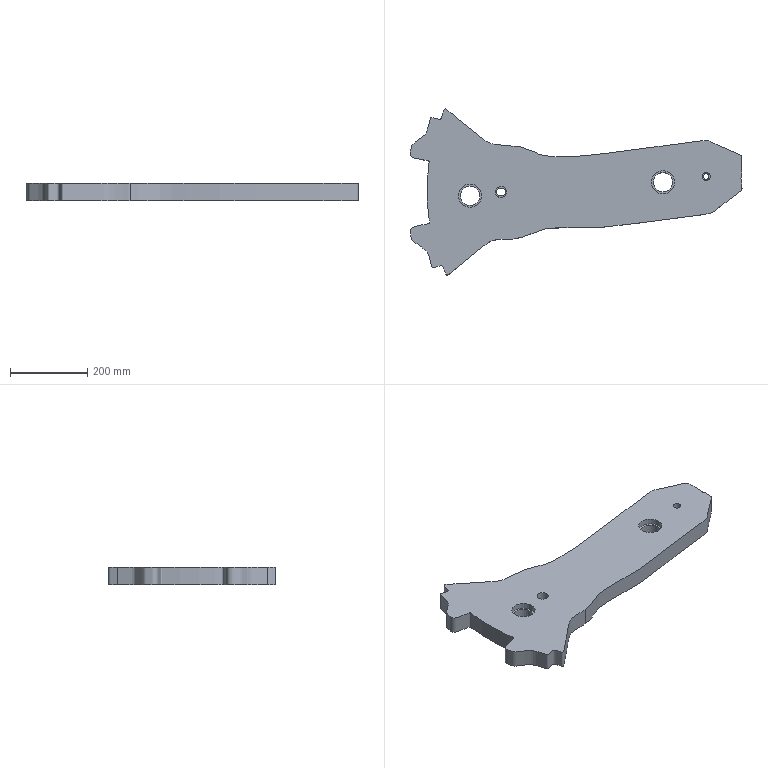Part | NX | features solid 2 | 1 solid | 29 faces | box 860.43 x 430.677 x 45 mm | volume 8766839 mm3 | cylinder 14 | plane 8 | cone 4 | spline 3 | commonest cylinder face diameters 12 x4 19 x2 50 x2 60 x2 14.1 x1 16 x1